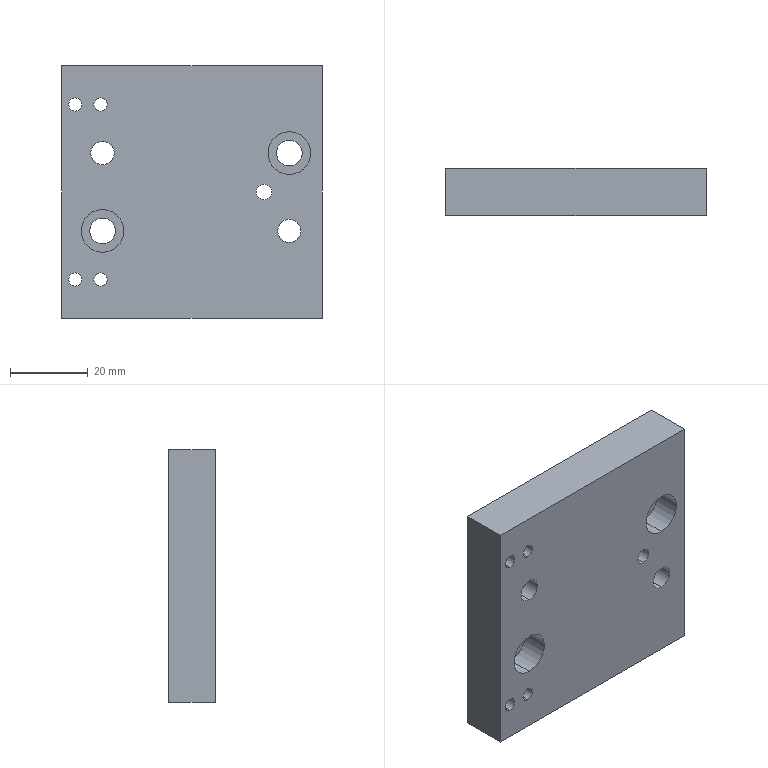Part | SolidWorks | features HoleWzd 3, Extrusion 1 | 1 solid | 42 faces | box 67 x 12 x 65 mm | volume 49086 mm3 | cylinder 30 | plane 12 | commonest cylinder face diameters 6 x12 3.4 x8 6.6 x4 11 x4 4 x2
STEP:
#1=CARTESIAN_POINT('',(25.,6.,-7.));
#2=VERTEX_POINT('',#1);
#3=CARTESIAN_POINT('',(25.,6.,-13.));
#4=VERTEX_POINT('',#3);
#5=CARTESIAN_POINT('',(25.,6.,-10.));
#6=DIRECTION('',(0.,-1.,0.));
#7=DIRECTION('',(0.,0.,-1.));
#8=AXIS2_PLACEMENT_3D('',#5,#6,#7);
#9=CIRCLE('',#8,3.);
#10=EDGE_CURVE('',#2,#4,#9,.T.);
#11=ORIENTED_EDGE('',*,*,#10,.F.);
#12=CARTESIAN_POINT('',(25.,-6.,-7.));
#13=VERTEX_POINT('',#12);
#14=CARTESIAN_POINT('',(25.,-6.,-7.));
#15=DIRECTION('',(0.,-1.,0.));
#16=VECTOR('',#15,1000.);
#17=LINE('',#14,#16);
#18=EDGE_CURVE('',#2,#13,#17,.T.);
#19=ORIENTED_EDGE('',*,*,#18,.T.);
#20=CARTESIAN_POINT('',(25.,-6.,-13.));
#21=VERTEX_POINT('',#20);
#22=CARTESIAN_POINT('',(25.,-6.,-10.));
#23=DIRECTION('',(0.,-1.,0.));
#24=DIRECTION('',(0.,0.,-1.));
#25=AXIS2_PLACEMENT_3D('',#22,#23,#24);
#26=CIRCLE('',#25,3.);
#27=EDGE_CURVE('',#13,#21,#26,.T.);
#28=ORIENTED_EDGE('',*,*,#27,.T.);
#29=CARTESIAN_POINT('',(25.,-6.,-13.));
#30=DIRECTION('',(0.,-1.,0.));
#31=VECTOR('',#30,1000.);
#32=LINE('',#29,#31);
#33=EDGE_CURVE('',#4,#21,#32,.T.);
#34=ORIENTED_EDGE('',*,*,#33,.F.);
#35=EDGE_LOOP('',(#11,#19,#28,#34));
#36=FACE_OUTER_BOUND('',#35,.T.);
#37=CARTESIAN_POINT('',(25.,-6.,-10.));
#38=DIRECTION('',(0.,-1.,0.));
#39=DIRECTION('',(0.,0.,-1.));
#40=AXIS2_PLACEMENT_3D('',#37,#38,#39);
#41=CYLINDRICAL_SURFACE('',#40,3.);
#42=ADVANCED_FACE('',(#36),#41,.F.);
#43=CARTESIAN_POINT('',(-23.,6.,13.));
#44=VERTEX_POINT('',#43);
#45=CARTESIAN_POINT('',(-23.,6.,7.));
#46=VERTEX_POINT('',#45);
#47=CARTESIAN_POINT('',(-23.,6.,10.));
#48=DIRECTION('',(0.,-1.,0.));
#49=DIRECTION('',(0.,0.,-1.));
#50=AXIS2_PLACEMENT_3D('',#47,#48,#49);
#51=CIRCLE('',#50,3.);
#52=EDGE_CURVE('',#44,#46,#51,.T.);
#53=ORIENTED_EDGE('',*,*,#52,.F.);
#54=CARTESIAN_POINT('',(-23.,-6.,13.));
#55=VERTEX_POINT('',#54);
#56=CARTESIAN_POINT('',(-23.,-6.,13.));
#57=DIRECTION('',(0.,-1.,0.));
#58=VECTOR('',#57,1000.);
#59=LINE('',#56,#58);
#60=EDGE_CURVE('',#44,#55,#59,.T.);
#61=ORIENTED_EDGE('',*,*,#60,.T.);
#62=CARTESIAN_POINT('',(-23.,-6.,7.));
#63=VERTEX_POINT('',#62);
#64=CARTESIAN_POINT('',(-23.,-6.,10.));
#65=DIRECTION('',(0.,-1.,0.));
#66=DIRECTION('',(0.,0.,-1.));
#67=AXIS2_PLACEMENT_3D('',#64,#65,#66);
#68=CIRCLE('',#67,3.);
#69=EDGE_CURVE('',#55,#63,#68,.T.);
#70=ORIENTED_EDGE('',*,*,#69,.T.);
#71=CARTESIAN_POINT('',(-23.,-6.,7.));
#72=DIRECTION('',(0.,-1.,0.));
#73=VECTOR('',#72,1000.);
#74=LINE('',#71,#73);
#75=EDGE_CURVE('',#46,#63,#74,.T.);
#76=ORIENTED_EDGE('',*,*,#75,.F.);
#77=EDGE_LOOP('',(#53,#61,#70,#76));
#78=FACE_OUTER_BOUND('',#77,.T.);
#79=CARTESIAN_POINT('',(-23.,-6.,10.));
#80=DIRECTION('',(0.,-1.,0.));
#81=DIRECTION('',(0.,0.,-1.));
#82=AXIS2_PLACEMENT_3D('',#79,#80,#81);
#83=CYLINDRICAL_SURFACE('',#82,3.);
#84=ADVANCED_FACE('',(#78),#83,.F.);
#85=CARTESIAN_POINT('',(-23.,0.8,-4.5));
#86=VERTEX_POINT('',#85);
#87=CARTESIAN_POINT('',(-23.,0.8,-15.5));
#88=VERTEX_POINT('',#87);
#89=CARTESIAN_POINT('',(-23.,0.8,-10.));
#90=DIRECTION('',(0.,-1.,0.));
#91=DIRECTION('',(0.,0.,-1.));
#92=AXIS2_PLACEMENT_3D('',#89,#90,#91);
#93=CIRCLE('',#92,5.5);
#94=EDGE_CURVE('',#86,#88,#93,.T.);
#95=ORIENTED_EDGE('',*,*,#94,.F.);
#96=CARTESIAN_POINT('',(-23.,-6.,-4.5));
#97=VERTEX_POINT('',#96);
#98=CARTESIAN_POINT('',(-23.,-6.,-4.5));
#99=DIRECTION('',(0.,-1.,0.));
#100=VECTOR('',#99,1000.);
#101=LINE('',#98,#100);
#102=EDGE_CURVE('',#86,#97,#101,.T.);
#103=ORIENTED_EDGE('',*,*,#102,.T.);
#104=CARTESIAN_POINT('',(-23.,-6.,-15.5));
#105=VERTEX_POINT('',#104);
#106=CARTESIAN_POINT('',(-23.,-6.,-10.));
#107=DIRECTION('',(0.,-1.,0.));
#108=DIRECTION('',(0.,0.,-1.));
#109=AXIS2_PLACEMENT_3D('',#106,#107,#108);
#110=CIRCLE('',#109,5.5);
#111=EDGE_CURVE('',#97,#105,#110,.T.);
#112=ORIENTED_EDGE('',*,*,#111,.T.);
#113=CARTESIAN_POINT('',(-23.,-6.,-15.5));
#114=DIRECTION('',(0.,-1.,0.));
#115=VECTOR('',#114,1000.);
#116=LINE('',#113,#115);
#117=EDGE_CURVE('',#88,#105,#116,.T.);
#118=ORIENTED_EDGE('',*,*,#117,.F.);
#119=EDGE_LOOP('',(#95,#103,#112,#118));
#120=FACE_OUTER_BOUND('',#119,.T.);
#121=CARTESIAN_POINT('',(-23.,-6.,-10.));
#122=DIRECTION('',(0.,-1.,0.));
#123=DIRECTION('',(0.,0.,-1.));
#124=AXIS2_PLACEMENT_3D('',#121,#122,#123);
#125=CYLINDRICAL_SURFACE('',#124,5.5);
#126=ADVANCED_FACE('',(#120),#125,.F.);
#127=CARTESIAN_POINT('',(-23.,6.,-6.7));
#128=VERTEX_POINT('',#127);
#129=CARTESIAN_POINT('',(-23.,6.,-13.3));
#130=VERTEX_POINT('',#129);
#131=CARTESIAN_POINT('',(-23.,6.,-10.));
#132=DIRECTION('',(0.,-1.,0.));
#133=DIRECTION('',(0.,0.,-1.));
#134=AXIS2_PLACEMENT_3D('',#131,#132,#133);
#135=CIRCLE('',#134,3.3);
#136=EDGE_CURVE('',#128,#130,#135,.T.);
#137=ORIENTED_EDGE('',*,*,#136,.F.);
#138=CARTESIAN_POINT('',(-23.,0.8,-6.7));
#139=VERTEX_POINT('',#138);
#140=CARTESIAN_POINT('',(-23.,-6.,-6.7));
#141=DIRECTION('',(0.,-1.,0.));
#142=VECTOR('',#141,1000.);
#143=LINE('',#140,#142);
#144=EDGE_CURVE('',#128,#139,#143,.T.);
#145=ORIENTED_EDGE('',*,*,#144,.T.);
#146=CARTESIAN_POINT('',(-23.,0.8,-13.3));
#147=VERTEX_POINT('',#146);
#148=CARTESIAN_POINT('',(-23.,0.8,-10.));
#149=DIRECTION('',(0.,-1.,0.));
#150=DIRECTION('',(0.,0.,-1.));
#151=AXIS2_PLACEMENT_3D('',#148,#149,#150);
#152=CIRCLE('',#151,3.3);
#153=EDGE_CURVE('',#139,#147,#152,.T.);
#154=ORIENTED_EDGE('',*,*,#153,.T.);
#155=CARTESIAN_POINT('',(-23.,-6.,-13.3));
#156=DIRECTION('',(0.,-1.,0.));
#157=VECTOR('',#156,1000.);
#158=LINE('',#155,#157);
#159=EDGE_CURVE('',#130,#147,#158,.T.);
#160=ORIENTED_EDGE('',*,*,#159,.F.);
#161=EDGE_LOOP('',(#137,#145,#154,#160));
#162=FACE_OUTER_BOUND('',#161,.T.);
#163=CARTESIAN_POINT('',(-23.,-6.,-10.));
#164=DIRECTION('',(0.,-1.,0.));
#165=DIRECTION('',(0.,0.,-1.));
#166=AXIS2_PLACEMENT_3D('',#163,#164,#165);
#167=CYLINDRICAL_SURFACE('',#166,3.3);
#168=ADVANCED_FACE('',(#162),#167,.F.);
#169=CARTESIAN_POINT('',(25.,0.8,15.5));
#170=VERTEX_POINT('',#169);
#171=CARTESIAN_POINT('',(25.,0.8,4.5));
#172=VERTEX_POINT('',#171);
#173=CARTESIAN_POINT('',(25.,0.8,10.));
#174=DIRECTION('',(0.,-1.,0.));
#175=DIRECTION('',(0.,0.,-1.));
#176=AXIS2_PLACEMENT_3D('',#173,#174,#175);
#177=CIRCLE('',#176,5.5);
#178=EDGE_CURVE('',#170,#172,#177,.T.);
#179=ORIENTED_EDGE('',*,*,#178,.F.);
#180=CARTESIAN_POINT('',(25.,-6.,15.5));
#181=VERTEX_POINT('',#180);
#182=CARTESIAN_POINT('',(25.,-6.,15.5));
#183=DIRECTION('',(0.,-1.,0.));
#184=VECTOR('',#183,1000.);
#185=LINE('',#182,#184);
#186=EDGE_CURVE('',#170,#181,#185,.T.);
#187=ORIENTED_EDGE('',*,*,#186,.T.);
#188=CARTESIAN_POINT('',(25.,-6.,4.5));
#189=VERTEX_POINT('',#188);
#190=CARTESIAN_POINT('',(25.,-6.,10.));
#191=DIRECTION('',(0.,-1.,0.));
#192=DIRECTION('',(0.,0.,-1.));
#193=AXIS2_PLACEMENT_3D('',#190,#191,#192);
#194=CIRCLE('',#193,5.5);
#195=EDGE_CURVE('',#181,#189,#194,.T.);
#196=ORIENTED_EDGE('',*,*,#195,.T.);
#197=CARTESIAN_POINT('',(25.,-6.,4.5));
#198=DIRECTION('',(0.,-1.,0.));
#199=VECTOR('',#198,1000.);
#200=LINE('',#197,#199);
#201=EDGE_CURVE('',#172,#189,#200,.T.);
#202=ORIENTED_EDGE('',*,*,#201,.F.);
#203=EDGE_LOOP('',(#179,#187,#196,#202));
#204=FACE_OUTER_BOUND('',#203,.T.);
#205=CARTESIAN_POINT('',(25.,-6.,10.));
#206=DIRECTION('',(0.,-1.,0.));
#207=DIRECTION('',(0.,0.,-1.));
#208=AXIS2_PLACEMENT_3D('',#205,#206,#207);
#209=CYLINDRICAL_SURFACE('',#208,5.5);
#210=ADVANCED_FACE('',(#204),#209,.F.);
#211=CARTESIAN_POINT('',(25.,6.,13.3));
#212=VERTEX_POINT('',#211);
#213=CARTESIAN_POINT('',(25.,6.,6.7));
#214=VERTEX_POINT('',#213);
#215=CARTESIAN_POINT('',(25.,6.,10.));
#216=DIRECTION('',(0.,-1.,0.));
#217=DIRECTION('',(0.,0.,-1.));
#218=AXIS2_PLACEMENT_3D('',#215,#216,#217);
#219=CIRCLE('',#218,3.3);
#220=EDGE_CURVE('',#212,#214,#219,.T.);
#221=ORIENTED_EDGE('',*,*,#220,.F.);
#222=CARTESIAN_POINT('',(25.,0.8,13.3));
#223=VERTEX_POINT('',#222);
#224=CARTESIAN_POINT('',(25.,-6.,13.3));
#225=DIRECTION('',(0.,-1.,0.));
#226=VECTOR('',#225,1000.);
#227=LINE('',#224,#226);
#228=EDGE_CURVE('',#212,#223,#227,.T.);
#229=ORIENTED_EDGE('',*,*,#228,.T.);
#230=CARTESIAN_POINT('',(25.,0.8,6.7));
#231=VERTEX_POINT('',#230);
#232=CARTESIAN_POINT('',(25.,0.8,10.));
#233=DIRECTION('',(0.,-1.,0.));
#234=DIRECTION('',(0.,0.,-1.));
#235=AXIS2_PLACEMENT_3D('',#232,#233,#234);
#236=CIRCLE('',#235,3.3);
#237=EDGE_CURVE('',#223,#231,#236,.T.);
#238=ORIENTED_EDGE('',*,*,#237,.T.);
#239=CARTESIAN_POINT('',(25.,-6.,6.7));
#240=DIRECTION('',(0.,-1.,0.));
#241=VECTOR('',#240,1000.);
#242=LINE('',#239,#241);
#243=EDGE_CURVE('',#214,#231,#242,.T.);
#244=ORIENTED_EDGE('',*,*,#243,.F.);
#245=EDGE_LOOP('',(#221,#229,#238,#244));
#246=FACE_OUTER_BOUND('',#245,.T.);
#247=CARTESIAN_POINT('',(25.,-6.,10.));
#248=DIRECTION('',(0.,-1.,0.));
#249=DIRECTION('',(0.,0.,-1.));
#250=AXIS2_PLACEMENT_3D('',#247,#248,#249);
#251=CYLINDRICAL_SURFACE('',#250,3.3);
#252=ADVANCED_FACE('',(#246),#251,.F.);
#253=CARTESIAN_POINT('',(-30.,2.6,19.5));
#254=VERTEX_POINT('',#253);
#255=CARTESIAN_POINT('',(-30.,2.6,25.5));
#256=VERTEX_POINT('',#255);
#257=CARTESIAN_POINT('',(-30.,2.6,22.5));
#258=DIRECTION('',(0.,1.,0.));
#259=DIRECTION('',(0.,0.,1.));
#260=AXIS2_PLACEMENT_3D('',#257,#258,#259);
#261=CIRCLE('',#260,3.);
#262=EDGE_CURVE('',#254,#256,#261,.T.);
#263=ORIENTED_EDGE('',*,*,#262,.F.);
#264=CARTESIAN_POINT('',(-30.,6.,19.5));
#265=VERTEX_POINT('',#264);
#266=CARTESIAN_POINT('',(-30.,6.,19.5));
#267=DIRECTION('',(0.,1.,0.));
#268=VECTOR('',#267,1000.);
#269=LINE('',#266,#268);
#270=EDGE_CURVE('',#254,#265,#269,.T.);
#271=ORIENTED_EDGE('',*,*,#270,.T.);
#272=CARTESIAN_POINT('',(-30.,6.,25.5));
#273=VERTEX_POINT('',#272);
#274=CARTESIAN_POINT('',(-30.,6.,22.5));
#275=DIRECTION('',(0.,1.,0.));
#276=DIRECTION('',(0.,0.,1.));
#277=AXIS2_PLACEMENT_3D('',#274,#275,#276);
#278=CIRCLE('',#277,3.);
#279=EDGE_CURVE('',#265,#273,#278,.T.);
#280=ORIENTED_EDGE('',*,*,#279,.T.);
#281=CARTESIAN_POINT('',(-30.,6.,25.5));
#282=DIRECTION('',(0.,1.,0.));
#283=VECTOR('',#282,1000.);
#284=LINE('',#281,#283);
#285=EDGE_CURVE('',#256,#273,#284,.T.);
#286=ORIENTED_EDGE('',*,*,#285,.F.);
#287=EDGE_LOOP('',(#263,#271,#280,#286));
#288=FACE_OUTER_BOUND('',#287,.T.);
#289=CARTESIAN_POINT('',(-30.,6.,22.5));
#290=DIRECTION('',(0.,1.,0.));
#291=DIRECTION('',(0.,0.,1.));
#292=AXIS2_PLACEMENT_3D('',#289,#290,#291);
#293=CYLINDRICAL_SURFACE('',#292,3.);
#294=ADVANCED_FACE('',(#288),#293,.F.);
#295=CARTESIAN_POINT('',(-30.,-6.,20.8));
#296=VERTEX_POINT('',#295);
#297=CARTESIAN_POINT('',(-30.,-6.,24.2));
#298=VERTEX_POINT('',#297);
#299=CARTESIAN_POINT('',(-30.,-6.,22.5));
#300=DIRECTION('',(0.,1.,0.));
#301=DIRECTION('',(0.,0.,1.));
#302=AXIS2_PLACEMENT_3D('',#299,#300,#301);
#303=CIRCLE('',#302,1.7);
#304=EDGE_CURVE('',#296,#298,#303,.T.);
#305=ORIENTED_EDGE('',*,*,#304,.F.);
#306=CARTESIAN_POINT('',(-30.,2.6,20.8));
#307=VERTEX_POINT('',#306);
#308=CARTESIAN_POINT('',(-30.,6.,20.8));
#309=DIRECTION('',(0.,1.,0.));
#310=VECTOR('',#309,1000.);
#311=LINE('',#308,#310);
#312=EDGE_CURVE('',#296,#307,#311,.T.);
#313=ORIENTED_EDGE('',*,*,#312,.T.);
#314=CARTESIAN_POINT('',(-30.,2.6,24.2));
#315=VERTEX_POINT('',#314);
#316=CARTESIAN_POINT('',(-30.,2.6,22.5));
#317=DIRECTION('',(0.,1.,0.));
#318=DIRECTION('',(0.,0.,1.));
#319=AXIS2_PLACEMENT_3D('',#316,#317,#318);
#320=CIRCLE('',#319,1.7);
#321=EDGE_CURVE('',#307,#315,#320,.T.);
#322=ORIENTED_EDGE('',*,*,#321,.T.);
#323=CARTESIAN_POINT('',(-30.,6.,24.2));
#324=DIRECTION('',(0.,1.,0.));
#325=VECTOR('',#324,1000.);
#326=LINE('',#323,#325);
#327=EDGE_CURVE('',#298,#315,#326,.T.);
#328=ORIENTED_EDGE('',*,*,#327,.F.);
#329=EDGE_LOOP('',(#305,#313,#322,#328));
#330=FACE_OUTER_BOUND('',#329,.T.);
#331=CARTESIAN_POINT('',(-30.,6.,22.5));
#332=DIRECTION('',(0.,1.,0.));
#333=DIRECTION('',(0.,0.,1.));
#334=AXIS2_PLACEMENT_3D('',#331,#332,#333);
#335=CYLINDRICAL_SURFACE('',#334,1.7);
#336=ADVANCED_FACE('',(#330),#335,.F.);
#337=CARTESIAN_POINT('',(-23.5,2.6,19.5));
#338=VERTEX_POINT('',#337);
#339=CARTESIAN_POINT('',(-23.5,2.6,25.5));
#340=VERTEX_POINT('',#339);
#341=CARTESIAN_POINT('',(-23.5,2.6,22.5));
#342=DIRECTION('',(0.,1.,0.));
#343=DIRECTION('',(0.,0.,1.));
#344=AXIS2_PLACEMENT_3D('',#341,#342,#343);
#345=CIRCLE('',#344,3.);
#346=EDGE_CURVE('',#338,#340,#345,.T.);
#347=ORIENTED_EDGE('',*,*,#346,.F.);
#348=CARTESIAN_POINT('',(-23.5,6.,19.5));
#349=VERTEX_POINT('',#348);
#350=CARTESIAN_POINT('',(-23.5,6.,19.5));
#351=DIRECTION('',(0.,1.,0.));
#352=VECTOR('',#351,1000.);
#353=LINE('',#350,#352);
#354=EDGE_CURVE('',#338,#349,#353,.T.);
#355=ORIENTED_EDGE('',*,*,#354,.T.);
#356=CARTESIAN_POINT('',(-23.5,6.,25.5));
#357=VERTEX_POINT('',#356);
#358=CARTESIAN_POINT('',(-23.5,6.,22.5));
#359=DIRECTION('',(0.,1.,0.));
#360=DIRECTION('',(0.,0.,1.));
#361=AXIS2_PLACEMENT_3D('',#358,#359,#360);
#362=CIRCLE('',#361,3.);
#363=EDGE_CURVE('',#349,#357,#362,.T.);
#364=ORIENTED_EDGE('',*,*,#363,.T.);
#365=CARTESIAN_POINT('',(-23.5,6.,25.5));
#366=DIRECTION('',(0.,1.,0.));
#367=VECTOR('',#366,1000.);
#368=LINE('',#365,#367);
#369=EDGE_CURVE('',#340,#357,#368,.T.);
#370=ORIENTED_EDGE('',*,*,#369,.F.);
#371=EDGE_LOOP('',(#347,#355,#364,#370));
#372=FACE_OUTER_BOUND('',#371,.T.);
#373=CARTESIAN_POINT('',(-23.5,6.,22.5));
#374=DIRECTION('',(0.,1.,0.));
#375=DIRECTION('',(0.,0.,1.));
#376=AXIS2_PLACEMENT_3D('',#373,#374,#375);
#377=CYLINDRICAL_SURFACE('',#376,3.);
#378=ADVANCED_FACE('',(#372),#377,.F.);
#379=CARTESIAN_POINT('',(-23.5,-6.,20.8));
#380=VERTEX_POINT('',#379);
#381=CARTESIAN_POINT('',(-23.5,-6.,24.2));
#382=VERTEX_POINT('',#381);
#383=CARTESIAN_POINT('',(-23.5,-6.,22.5));
#384=DIRECTION('',(0.,1.,0.));
#385=DIRECTION('',(0.,0.,1.));
#386=AXIS2_PLACEMENT_3D('',#383,#384,#385);
#387=CIRCLE('',#386,1.7);
#388=EDGE_CURVE('',#380,#382,#387,.T.);
#389=ORIENTED_EDGE('',*,*,#388,.F.);
#390=CARTESIAN_POINT('',(-23.5,2.6,20.8));
#391=VERTEX_POINT('',#390);
#392=CARTESIAN_POINT('',(-23.5,6.,20.8));
#393=DIRECTION('',(0.,1.,0.));
#394=VECTOR('',#393,1000.);
#395=LINE('',#392,#394);
#396=EDGE_CURVE('',#380,#391,#395,.T.);
#397=ORIENTED_EDGE('',*,*,#396,.T.);
#398=CARTESIAN_POINT('',(-23.5,2.6,24.2));
#399=VERTEX_POINT('',#398);
#400=CARTESIAN_POINT('',(-23.5,2.6,22.5));
#401=DIRECTION('',(0.,1.,0.));
#402=DIRECTION('',(0.,0.,1.));
#403=AXIS2_PLACEMENT_3D('',#400,#401,#402);
#404=CIRCLE('',#403,1.7);
#405=EDGE_CURVE('',#391,#399,#404,.T.);
#406=ORIENTED_EDGE('',*,*,#405,.T.);
#407=CARTESIAN_POINT('',(-23.5,6.,24.2));
#408=DIRECTION('',(0.,1.,0.));
#409=VECTOR('',#408,1000.);
#410=LINE('',#407,#409);
#411=EDGE_CURVE('',#382,#399,#410,.T.);
#412=ORIENTED_EDGE('',*,*,#411,.F.);
#413=EDGE_LOOP('',(#389,#397,#406,#412));
#414=FACE_OUTER_BOUND('',#413,.T.);
#415=CARTESIAN_POINT('',(-23.5,6.,22.5));
#416=DIRECTION('',(0.,1.,0.));
#417=DIRECTION('',(0.,0.,1.));
#418=AXIS2_PLACEMENT_3D('',#415,#416,#417);
#419=CYLINDRICAL_SURFACE('',#418,1.7);
#420=ADVANCED_FACE('',(#414),#419,.F.);
#421=CARTESIAN_POINT('',(-23.5,2.6,-25.5));
#422=VERTEX_POINT('',#421);
#423=CARTESIAN_POINT('',(-23.5,2.6,-19.5));
#424=VERTEX_POINT('',#423);
#425=CARTESIAN_POINT('',(-23.5,2.6,-22.5));
#426=DIRECTION('',(0.,1.,0.));
#427=DIRECTION('',(0.,0.,1.));
#428=AXIS2_PLACEMENT_3D('',#425,#426,#427);
#429=CIRCLE('',#428,3.);
#430=EDGE_CURVE('',#422,#424,#429,.T.);
#431=ORIENTED_EDGE('',*,*,#430,.F.);
#432=CARTESIAN_POINT('',(-23.5,6.,-25.5));
#433=VERTEX_POINT('',#432);
#434=CARTESIAN_POINT('',(-23.5,6.,-25.5));
#435=DIRECTION('',(0.,1.,0.));
#436=VECTOR('',#435,1000.);
#437=LINE('',#434,#436);
#438=EDGE_CURVE('',#422,#433,#437,.T.);
#439=ORIENTED_EDGE('',*,*,#438,.T.);
#440=CARTESIAN_POINT('',(-23.5,6.,-19.5));
#441=VERTEX_POINT('',#440);
#442=CARTESIAN_POINT('',(-23.5,6.,-22.5));
#443=DIRECTION('',(0.,1.,0.));
#444=DIRECTION('',(0.,0.,1.));
#445=AXIS2_PLACEMENT_3D('',#442,#443,#444);
#446=CIRCLE('',#445,3.);
#447=EDGE_CURVE('',#433,#441,#446,.T.);
#448=ORIENTED_EDGE('',*,*,#447,.T.);
#449=CARTESIAN_POINT('',(-23.5,6.,-19.5));
#450=DIRECTION('',(0.,1.,0.));
#451=VECTOR('',#450,1000.);
#452=LINE('',#449,#451);
#453=EDGE_CURVE('',#424,#441,#452,.T.);
#454=ORIENTED_EDGE('',*,*,#453,.F.);
#455=EDGE_LOOP('',(#431,#439,#448,#454));
#456=FACE_OUTER_BOUND('',#455,.T.);
#457=CARTESIAN_POINT('',(-23.5,6.,-22.5));
#458=DIRECTION('',(0.,1.,0.));
#459=DIRECTION('',(0.,0.,1.));
#460=AXIS2_PLACEMENT_3D('',#457,#458,#459);
#461=CYLINDRICAL_SURFACE('',#460,3.);
#462=ADVANCED_FACE('',(#456),#461,.F.);
#463=CARTESIAN_POINT('',(-23.5,-6.,-24.2));
#464=VERTEX_POINT('',#463);
#465=CARTESIAN_POINT('',(-23.5,-6.,-20.8));
#466=VERTEX_POINT('',#465);
#467=CARTESIAN_POINT('',(-23.5,-6.,-22.5));
#468=DIRECTION('',(0.,1.,0.));
#469=DIRECTION('',(0.,0.,1.));
#470=AXIS2_PLACEMENT_3D('',#467,#468,#469);
#471=CIRCLE('',#470,1.7);
#472=EDGE_CURVE('',#464,#466,#471,.T.);
#473=ORIENTED_EDGE('',*,*,#472,.F.);
#474=CARTESIAN_POINT('',(-23.5,2.6,-24.2));
#475=VERTEX_POINT('',#474);
#476=CARTESIAN_POINT('',(-23.5,6.,-24.2));
#477=DIRECTION('',(0.,1.,0.));
#478=VECTOR('',#477,1000.);
#479=LINE('',#476,#478);
#480=EDGE_CURVE('',#464,#475,#479,.T.);
#481=ORIENTED_EDGE('',*,*,#480,.T.);
#482=CARTESIAN_POINT('',(-23.5,2.6,-20.8));
#483=VERTEX_POINT('',#482);
#484=CARTESIAN_POINT('',(-23.5,2.6,-22.5));
#485=DIRECTION('',(0.,1.,0.));
#486=DIRECTION('',(0.,0.,1.));
#487=AXIS2_PLACEMENT_3D('',#484,#485,#486);
#488=CIRCLE('',#487,1.7);
#489=EDGE_CURVE('',#475,#483,#488,.T.);
#490=ORIENTED_EDGE('',*,*,#489,.T.);
#491=CARTESIAN_POINT('',(-23.5,6.,-20.8));
#492=DIRECTION('',(0.,1.,0.));
#493=VECTOR('',#492,1000.);
#494=LINE('',#491,#493);
#495=EDGE_CURVE('',#466,#483,#494,.T.);
#496=ORIENTED_EDGE('',*,*,#495,.F.);
#497=EDGE_LOOP('',(#473,#481,#490,#496));
#498=FACE_OUTER_BOUND('',#497,.T.);
#499=CARTESIAN_POINT('',(-23.5,6.,-22.5));
#500=DIRECTION('',(0.,1.,0.));
#501=DIRECTION('',(0.,0.,1.));
#502=AXIS2_PLACEMENT_3D('',#499,#500,#501);
#503=CYLINDRICAL_SURFACE('',#502,1.7);
#504=ADVANCED_FACE('',(#498),#503,.F.);
#505=CARTESIAN_POINT('',(-30.,2.6,-25.5));
#506=VERTEX_POINT('',#505);
#507=CARTESIAN_POINT('',(-30.,2.6,-19.5));
#508=VERTEX_POINT('',#507);
#509=CARTESIAN_POINT('',(-30.,2.6,-22.5));
#510=DIRECTION('',(0.,1.,0.));
#511=DIRECTION('',(0.,0.,1.));
#512=AXIS2_PLACEMENT_3D('',#509,#510,#511);
#513=CIRCLE('',#512,3.);
#514=EDGE_CURVE('',#506,#508,#513,.T.);
#515=ORIENTED_EDGE('',*,*,#514,.F.);
#516=CARTESIAN_POINT('',(-30.,6.,-25.5));
#517=VERTEX_POINT('',#516);
#518=CARTESIAN_POINT('',(-30.,6.,-25.5));
#519=DIRECTION('',(0.,1.,0.));
#520=VECTOR('',#519,1000.);
#521=LINE('',#518,#520);
#522=EDGE_CURVE('',#506,#517,#521,.T.);
#523=ORIENTED_EDGE('',*,*,#522,.T.);
#524=CARTESIAN_POINT('',(-30.,6.,-19.5));
#525=VERTEX_POINT('',#524);
#526=CARTESIAN_POINT('',(-30.,6.,-22.5));
#527=DIRECTION('',(0.,1.,0.));
#528=DIRECTION('',(0.,0.,1.));
#529=AXIS2_PLACEMENT_3D('',#526,#527,#528);
#530=CIRCLE('',#529,3.);
#531=EDGE_CURVE('',#517,#525,#530,.T.);
#532=ORIENTED_EDGE('',*,*,#531,.T.);
#533=CARTESIAN_POINT('',(-30.,6.,-19.5));
#534=DIRECTION('',(0.,1.,0.));
#535=VECTOR('',#534,1000.);
#536=LINE('',#533,#535);
#537=EDGE_CURVE('',#508,#525,#536,.T.);
#538=ORIENTED_EDGE('',*,*,#537,.F.);
#539=EDGE_LOOP('',(#515,#523,#532,#538));
#540=FACE_OUTER_BOUND('',#539,.T.);
#541=CARTESIAN_POINT('',(-30.,6.,-22.5));
#542=DIRECTION('',(0.,1.,0.));
#543=DIRECTION('',(0.,0.,1.));
#544=AXIS2_PLACEMENT_3D('',#541,#542,#543);
#545=CYLINDRICAL_SURFACE('',#544,3.);
#546=ADVANCED_FACE('',(#540),#545,.F.);
#547=CARTESIAN_POINT('',(-30.,-6.,-24.2));
#548=VERTEX_POINT('',#547);
#549=CARTESIAN_POINT('',(-30.,-6.,-20.8));
#550=VERTEX_POINT('',#549);
#551=CARTESIAN_POINT('',(-30.,-6.,-22.5));
#552=DIRECTION('',(0.,1.,0.));
#553=DIRECTION('',(0.,0.,1.));
#554=AXIS2_PLACEMENT_3D('',#551,#552,#553);
#555=CIRCLE('',#554,1.7);
#556=EDGE_CURVE('',#548,#550,#555,.T.);
#557=ORIENTED_EDGE('',*,*,#556,.F.);
#558=CARTESIAN_POINT('',(-30.,2.6,-24.2));
#559=VERTEX_POINT('',#558);
#560=CARTESIAN_POINT('',(-30.,6.,-24.2));
#561=DIRECTION('',(0.,1.,0.));
#562=VECTOR('',#561,1000.);
#563=LINE('',#560,#562);
#564=EDGE_CURVE('',#548,#559,#563,.T.);
#565=ORIENTED_EDGE('',*,*,#564,.T.);
#566=CARTESIAN_POINT('',(-30.,2.6,-20.8));
#567=VERTEX_POINT('',#566);
#568=CARTESIAN_POINT('',(-30.,2.6,-22.5));
#569=DIRECTION('',(0.,1.,0.));
#570=DIRECTION('',(0.,0.,1.));
#571=AXIS2_PLACEMENT_3D('',#568,#569,#570);
#572=CIRCLE('',#571,1.7);
#573=EDGE_CURVE('',#559,#567,#572,.T.);
#574=ORIENTED_EDGE('',*,*,#573,.T.);
#575=CARTESIAN_POINT('',(-30.,6.,-20.8));
#576=DIRECTION('',(0.,1.,0.));
#577=VECTOR('',#576,1000.);
#578=LINE('',#575,#577);
#579=EDGE_CURVE('',#550,#567,#578,.T.);
#580=ORIENTED_EDGE('',*,*,#579,.F.);
#581=EDGE_LOOP('',(#557,#565,#574,#580));
#582=FACE_OUTER_BOUND('',#581,.T.);
#583=CARTESIAN_POINT('',(-30.,6.,-22.5));
#584=DIRECTION('',(0.,1.,0.));
#585=DIRECTION('',(0.,0.,1.));
#586=AXIS2_PLACEMENT_3D('',#583,#584,#585);
#587=CYLINDRICAL_SURFACE('',#586,1.7);
#588=ADVANCED_FACE('',(#582),#587,.F.);
#589=CARTESIAN_POINT('',(18.5,6.,-2.));
#590=VERTEX_POINT('',#589);
#591=CARTESIAN_POINT('',(18.5,6.,2.));
#592=VERTEX_POINT('',#591);
#593=CARTESIAN_POINT('',(18.5,6.,0.));
#594=DIRECTION('',(0.,1.,0.));
#595=DIRECTION('',(0.,0.,1.));
#596=AXIS2_PLACEMENT_3D('',#593,#594,#595);
#597=CIRCLE('',#596,2.);
#598=EDGE_CURVE('',#590,#592,#597,.T.);
#599=ORIENTED_EDGE('',*,*,#598,.T.);
#600=CARTESIAN_POINT('',(18.5,-6.,2.));
#601=VERTEX_POINT('',#600);
#602=CARTESIAN_POINT('',(18.5,6.,2.));
#603=DIRECTION('',(0.,-1.,0.));
#604=VECTOR('',#603,1000.);
#605=LINE('',#602,#604);
#606=EDGE_CURVE('',#592,#601,#605,.T.);
#607=ORIENTED_EDGE('',*,*,#606,.T.);
#608=CARTESIAN_POINT('',(18.5,-6.,-2.));
#609=VERTEX_POINT('',#608);
#610=CARTESIAN_POINT('',(18.5,-6.,0.));
#611=DIRECTION('',(0.,1.,0.));
#612=DIRECTION('',(0.,0.,1.));
#613=AXIS2_PLACEMENT_3D('',#610,#611,#612);
#614=CIRCLE('',#613,2.);
#615=EDGE_CURVE('',#609,#601,#614,.T.);
#616=ORIENTED_EDGE('',*,*,#615,.F.);
#617=CARTESIAN_POINT('',(18.5,6.,-2.));
#618=DIRECTION('',(0.,-1.,0.));
#619=VECTOR('',#618,1000.);
#620=LINE('',#617,#619);
#621=EDGE_CURVE('',#590,#609,#620,.T.);
#622=ORIENTED_EDGE('',*,*,#621,.F.);
#623=EDGE_LOOP('',(#599,#607,#616,#622));
#624=FACE_OUTER_BOUND('',#623,.T.);
#625=CARTESIAN_POINT('',(18.5,6.,0.));
#626=DIRECTION('',(0.,-1.,0.));
#627=DIRECTION('',(0.,0.,-1.));
#628=AXIS2_PLACEMENT_3D('',#625,#626,#627);
#629=CYLINDRICAL_SURFACE('',#628,2.);
#630=ADVANCED_FACE('',(#624),#629,.F.);
#631=CARTESIAN_POINT('',(25.,6.,-10.));
#632=DIRECTION('',(0.,-1.,0.));
#633=DIRECTION('',(0.,0.,-1.));
#634=AXIS2_PLACEMENT_3D('',#631,#632,#633);
#635=CIRCLE('',#634,3.);
#636=EDGE_CURVE('',#4,#2,#635,.T.);
#637=ORIENTED_EDGE('',*,*,#636,.T.);
#638=ORIENTED_EDGE('',*,*,#10,.T.);
#639=EDGE_LOOP('',(#637,#638));
#640=FACE_BOUND('',#639,.T.);
#641=CARTESIAN_POINT('',(-23.,6.,10.));
#642=DIRECTION('',(0.,-1.,0.));
#643=DIRECTION('',(0.,0.,-1.));
#644=AXIS2_PLACEMENT_3D('',#641,#642,#643);
#645=CIRCLE('',#644,3.);
#646=EDGE_CURVE('',#46,#44,#645,.T.);
#647=ORIENTED_EDGE('',*,*,#646,.T.);
#648=ORIENTED_EDGE('',*,*,#52,.T.);
#649=EDGE_LOOP('',(#647,#648));
#650=FACE_BOUND('',#649,.T.);
#651=CARTESIAN_POINT('',(-23.,6.,-10.));
#652=DIRECTION('',(0.,-1.,0.));
#653=DIRECTION('',(0.,0.,-1.));
#654=AXIS2_PLACEMENT_3D('',#651,#652,#653);
#655=CIRCLE('',#654,3.3);
#656=EDGE_CURVE('',#130,#128,#655,.T.);
#657=ORIENTED_EDGE('',*,*,#656,.T.);
#658=ORIENTED_EDGE('',*,*,#136,.T.);
#659=EDGE_LOOP('',(#657,#658));
#660=FACE_BOUND('',#659,.T.);
#661=CARTESIAN_POINT('',(25.,6.,10.));
#662=DIRECTION('',(0.,-1.,0.));
#663=DIRECTION('',(0.,0.,-1.));
#664=AXIS2_PLACEMENT_3D('',#661,#662,#663);
#665=CIRCLE('',#664,3.3);
#666=EDGE_CURVE('',#214,#212,#665,.T.);
#667=ORIENTED_EDGE('',*,*,#666,.T.);
#668=ORIENTED_EDGE('',*,*,#220,.T.);
#669=EDGE_LOOP('',(#667,#668));
#670=FACE_BOUND('',#669,.T.);
#671=CARTESIAN_POINT('',(-30.,6.,22.5));
#672=DIRECTION('',(0.,1.,0.));
#673=DIRECTION('',(0.,0.,1.));
#674=AXIS2_PLACEMENT_3D('',#671,#672,#673);
#675=CIRCLE('',#674,3.);
#676=EDGE_CURVE('',#273,#265,#675,.T.);
#677=ORIENTED_EDGE('',*,*,#676,.F.);
#678=ORIENTED_EDGE('',*,*,#279,.F.);
#679=EDGE_LOOP('',(#677,#678));
#680=FACE_BOUND('',#679,.T.);
#681=CARTESIAN_POINT('',(-23.5,6.,22.5));
#682=DIRECTION('',(0.,1.,0.));
#683=DIRECTION('',(0.,0.,1.));
#684=AXIS2_PLACEMENT_3D('',#681,#682,#683);
#685=CIRCLE('',#684,3.);
#686=EDGE_CURVE('',#357,#349,#685,.T.);
#687=ORIENTED_EDGE('',*,*,#686,.F.);
#688=ORIENTED_EDGE('',*,*,#363,.F.);
#689=EDGE_LOOP('',(#687,#688));
#690=FACE_BOUND('',#689,.T.);
#691=CARTESIAN_POINT('',(-23.5,6.,-22.5));
#692=DIRECTION('',(0.,1.,0.));
#693=DIRECTION('',(0.,0.,1.));
#694=AXIS2_PLACEMENT_3D('',#691,#692,#693);
#695=CIRCLE('',#694,3.);
#696=EDGE_CURVE('',#441,#433,#695,.T.);
#697=ORIENTED_EDGE('',*,*,#696,.F.);
#698=ORIENTED_EDGE('',*,*,#447,.F.);
#699=EDGE_LOOP('',(#697,#698));
#700=FACE_BOUND('',#699,.T.);
#701=CARTESIAN_POINT('',(33.5,6.,32.5));
#702=VERTEX_POINT('',#701);
#703=CARTESIAN_POINT('',(33.5,6.,-32.5));
#704=VERTEX_POINT('',#703);
#705=CARTESIAN_POINT('',(33.5,6.,32.5));
#706=DIRECTION('',(0.,0.,-1.));
#707=VECTOR('',#706,1000.);
#708=LINE('',#705,#707);
#709=EDGE_CURVE('',#702,#704,#708,.T.);
#710=ORIENTED_EDGE('',*,*,#709,.T.);
#711=CARTESIAN_POINT('',(-33.5,6.,-32.5));
#712=VERTEX_POINT('',#711);
#713=CARTESIAN_POINT('',(-33.5,6.,-32.5));
#714=DIRECTION('',(-1.,0.,0.));
#715=VECTOR('',#714,1000.);
#716=LINE('',#713,#715);
#717=EDGE_CURVE('',#704,#712,#716,.T.);
#718=ORIENTED_EDGE('',*,*,#717,.T.);
#719=CARTESIAN_POINT('',(-33.5,6.,32.5));
#720=VERTEX_POINT('',#719);
#721=CARTESIAN_POINT('',(-33.5,6.,32.5));
#722=DIRECTION('',(0.,0.,1.));
#723=VECTOR('',#722,1000.);
#724=LINE('',#721,#723);
#725=EDGE_CURVE('',#712,#720,#724,.T.);
#726=ORIENTED_EDGE('',*,*,#725,.T.);
#727=CARTESIAN_POINT('',(-33.5,6.,32.5));
#728=DIRECTION('',(1.,0.,0.));
#729=VECTOR('',#728,1000.);
#730=LINE('',#727,#729);
#731=EDGE_CURVE('',#720,#702,#730,.T.);
#732=ORIENTED_EDGE('',*,*,#731,.T.);
#733=EDGE_LOOP('',(#710,#718,#726,#732));
#734=FACE_OUTER_BOUND('',#733,.T.);
#735=ORIENTED_EDGE('',*,*,#598,.F.);
#736=CARTESIAN_POINT('',(18.5,6.,0.));
#737=DIRECTION('',(0.,1.,0.));
#738=DIRECTION('',(0.,0.,1.));
#739=AXIS2_PLACEMENT_3D('',#736,#737,#738);
#740=CIRCLE('',#739,2.);
#741=EDGE_CURVE('',#592,#590,#740,.T.);
#742=ORIENTED_EDGE('',*,*,#741,.F.);
#743=EDGE_LOOP('',(#735,#742));
#744=FACE_BOUND('',#743,.T.);
#745=CARTESIAN_POINT('',(-30.,6.,-22.5));
#746=DIRECTION('',(0.,1.,0.));
#747=DIRECTION('',(0.,0.,1.));
#748=AXIS2_PLACEMENT_3D('',#745,#746,#747);
#749=CIRCLE('',#748,3.);
#750=EDGE_CURVE('',#525,#517,#749,.T.);
#751=ORIENTED_EDGE('',*,*,#750,.F.);
#752=ORIENTED_EDGE('',*,*,#531,.F.);
#753=EDGE_LOOP('',(#751,#752));
#754=FACE_BOUND('',#753,.T.);
#755=CARTESIAN_POINT('',(0.,6.,0.));
#756=DIRECTION('',(0.,-1.,0.));
#757=DIRECTION('',(0.,0.,-1.));
#758=AXIS2_PLACEMENT_3D('',#755,#756,#757);
#759=PLANE('',#758);
#760=ADVANCED_FACE('',(#640,#650,#660,#670,#680,#690,#700,#734,#744,#754),#759,.F.);
#761=CARTESIAN_POINT('',(25.,-6.,-10.));
#762=DIRECTION('',(0.,-1.,0.));
#763=DIRECTION('',(0.,0.,-1.));
#764=AXIS2_PLACEMENT_3D('',#761,#762,#763);
#765=CIRCLE('',#764,3.);
#766=EDGE_CURVE('',#21,#13,#765,.T.);
#767=ORIENTED_EDGE('',*,*,#766,.F.);
#768=ORIENTED_EDGE('',*,*,#27,.F.);
#769=EDGE_LOOP('',(#767,#768));
#770=FACE_BOUND('',#769,.T.);
#771=CARTESIAN_POINT('',(-23.,-6.,10.));
#772=DIRECTION('',(0.,-1.,0.));
#773=DIRECTION('',(0.,0.,-1.));
#774=AXIS2_PLACEMENT_3D('',#771,#772,#773);
#775=CIRCLE('',#774,3.);
#776=EDGE_CURVE('',#63,#55,#775,.T.);
#777=ORIENTED_EDGE('',*,*,#776,.F.);
#778=ORIENTED_EDGE('',*,*,#69,.F.);
#779=EDGE_LOOP('',(#777,#778));
#780=FACE_BOUND('',#779,.T.);
#781=CARTESIAN_POINT('',(-23.,-6.,-10.));
#782=DIRECTION('',(0.,-1.,0.));
#783=DIRECTION('',(0.,0.,-1.));
#784=AXIS2_PLACEMENT_3D('',#781,#782,#783);
#785=CIRCLE('',#784,5.5);
#786=EDGE_CURVE('',#105,#97,#785,.T.);
#787=ORIENTED_EDGE('',*,*,#786,.F.);
#788=ORIENTED_EDGE('',*,*,#111,.F.);
#789=EDGE_LOOP('',(#787,#788));
#790=FACE_BOUND('',#789,.T.);
#791=CARTESIAN_POINT('',(25.,-6.,10.));
#792=DIRECTION('',(0.,-1.,0.));
#793=DIRECTION('',(0.,0.,-1.));
#794=AXIS2_PLACEMENT_3D('',#791,#792,#793);
#795=CIRCLE('',#794,5.5);
#796=EDGE_CURVE('',#189,#181,#795,.T.);
#797=ORIENTED_EDGE('',*,*,#796,.F.);
#798=ORIENTED_EDGE('',*,*,#195,.F.);
#799=EDGE_LOOP('',(#797,#798));
#800=FACE_BOUND('',#799,.T.);
#801=CARTESIAN_POINT('',(-30.,-6.,22.5));
#802=DIRECTION('',(0.,1.,0.));
#803=DIRECTION('',(0.,0.,1.));
#804=AXIS2_PLACEMENT_3D('',#801,#802,#803);
#805=CIRCLE('',#804,1.7);
#806=EDGE_CURVE('',#298,#296,#805,.T.);
#807=ORIENTED_EDGE('',*,*,#806,.T.);
#808=ORIENTED_EDGE('',*,*,#304,.T.);
#809=EDGE_LOOP('',(#807,#808));
#810=FACE_BOUND('',#809,.T.);
#811=CARTESIAN_POINT('',(-23.5,-6.,22.5));
#812=DIRECTION('',(0.,1.,0.));
#813=DIRECTION('',(0.,0.,1.));
#814=AXIS2_PLACEMENT_3D('',#811,#812,#813);
#815=CIRCLE('',#814,1.7);
#816=EDGE_CURVE('',#382,#380,#815,.T.);
#817=ORIENTED_EDGE('',*,*,#816,.T.);
#818=ORIENTED_EDGE('',*,*,#388,.T.);
#819=EDGE_LOOP('',(#817,#818));
#820=FACE_BOUND('',#819,.T.);
#821=CARTESIAN_POINT('',(-23.5,-6.,-22.5));
#822=DIRECTION('',(0.,1.,0.));
#823=DIRECTION('',(0.,0.,1.));
#824=AXIS2_PLACEMENT_3D('',#821,#822,#823);
#825=CIRCLE('',#824,1.7);
#826=EDGE_CURVE('',#466,#464,#825,.T.);
#827=ORIENTED_EDGE('',*,*,#826,.T.);
#828=ORIENTED_EDGE('',*,*,#472,.T.);
#829=EDGE_LOOP('',(#827,#828));
#830=FACE_BOUND('',#829,.T.);
#831=CARTESIAN_POINT('',(-30.,-6.,-22.5));
#832=DIRECTION('',(0.,1.,0.));
#833=DIRECTION('',(0.,0.,1.));
#834=AXIS2_PLACEMENT_3D('',#831,#832,#833);
#835=CIRCLE('',#834,1.7);
#836=EDGE_CURVE('',#550,#548,#835,.T.);
#837=ORIENTED_EDGE('',*,*,#836,.T.);
#838=ORIENTED_EDGE('',*,*,#556,.T.);
#839=EDGE_LOOP('',(#837,#838));
#840=FACE_BOUND('',#839,.T.);
#841=CARTESIAN_POINT('',(33.5,-6.,32.5));
#842=VERTEX_POINT('',#841);
#843=CARTESIAN_POINT('',(33.5,-6.,-32.5));
#844=VERTEX_POINT('',#843);
#845=CARTESIAN_POINT('',(33.5,-6.,32.5));
#846=DIRECTION('',(0.,0.,-1.));
#847=VECTOR('',#846,1000.);
#848=LINE('',#845,#847);
#849=EDGE_CURVE('',#842,#844,#848,.T.);
#850=ORIENTED_EDGE('',*,*,#849,.F.);
#851=CARTESIAN_POINT('',(-33.5,-6.,32.5));
#852=VERTEX_POINT('',#851);
#853=CARTESIAN_POINT('',(-33.5,-6.,32.5));
#854=DIRECTION('',(1.,0.,0.));
#855=VECTOR('',#854,1000.);
#856=LINE('',#853,#855);
#857=EDGE_CURVE('',#852,#842,#856,.T.);
#858=ORIENTED_EDGE('',*,*,#857,.F.);
#859=CARTESIAN_POINT('',(-33.5,-6.,-32.5));
#860=VERTEX_POINT('',#859);
#861=CARTESIAN_POINT('',(-33.5,-6.,32.5));
#862=DIRECTION('',(0.,0.,1.));
#863=VECTOR('',#862,1000.);
#864=LINE('',#861,#863);
#865=EDGE_CURVE('',#860,#852,#864,.T.);
#866=ORIENTED_EDGE('',*,*,#865,.F.);
#867=CARTESIAN_POINT('',(-33.5,-6.,-32.5));
#868=DIRECTION('',(-1.,0.,0.));
#869=VECTOR('',#868,1000.);
#870=LINE('',#867,#869);
#871=EDGE_CURVE('',#844,#860,#870,.T.);
#872=ORIENTED_EDGE('',*,*,#871,.F.);
#873=EDGE_LOOP('',(#850,#858,#866,#872));
#874=FACE_OUTER_BOUND('',#873,.T.);
#875=ORIENTED_EDGE('',*,*,#615,.T.);
#876=CARTESIAN_POINT('',(18.5,-6.,0.));
#877=DIRECTION('',(0.,1.,0.));
#878=DIRECTION('',(0.,0.,1.));
#879=AXIS2_PLACEMENT_3D('',#876,#877,#878);
#880=CIRCLE('',#879,2.);
#881=EDGE_CURVE('',#601,#609,#880,.T.);
#882=ORIENTED_EDGE('',*,*,#881,.T.);
#883=EDGE_LOOP('',(#875,#882));
#884=FACE_BOUND('',#883,.T.);
#885=CARTESIAN_POINT('',(0.,-6.,0.));
#886=DIRECTION('',(0.,-1.,0.));
#887=DIRECTION('',(0.,0.,-1.));
#888=AXIS2_PLACEMENT_3D('',#885,#886,#887);
#889=PLANE('',#888);
#890=ADVANCED_FACE('',(#770,#780,#790,#800,#810,#820,#830,#840,#874,#884),#889,.T.);
#891=ORIENTED_EDGE('',*,*,#849,.T.);
#892=CARTESIAN_POINT('',(33.5,6.,-32.5));
#893=DIRECTION('',(0.,-1.,0.));
#894=VECTOR('',#893,1000.);
#895=LINE('',#892,#894);
#896=EDGE_CURVE('',#704,#844,#895,.T.);
#897=ORIENTED_EDGE('',*,*,#896,.F.);
#898=ORIENTED_EDGE('',*,*,#709,.F.);
#899=CARTESIAN_POINT('',(33.5,6.,32.5));
#900=DIRECTION('',(0.,-1.,0.));
#901=VECTOR('',#900,1000.);
#902=LINE('',#899,#901);
#903=EDGE_CURVE('',#702,#842,#902,.T.);
#904=ORIENTED_EDGE('',*,*,#903,.T.);
#905=EDGE_LOOP('',(#891,#897,#898,#904));
#906=FACE_OUTER_BOUND('',#905,.T.);
#907=CARTESIAN_POINT('',(33.5,6.,32.5));
#908=DIRECTION('',(-1.,0.,0.));
#909=DIRECTION('',(0.,0.,1.));
#910=AXIS2_PLACEMENT_3D('',#907,#908,#909);
#911=PLANE('',#910);
#912=ADVANCED_FACE('',(#906),#911,.F.);
#913=ORIENTED_EDGE('',*,*,#871,.T.);
#914=CARTESIAN_POINT('',(-33.5,6.,-32.5));
#915=DIRECTION('',(0.,-1.,0.));
#916=VECTOR('',#915,1000.);
#917=LINE('',#914,#916);
#918=EDGE_CURVE('',#712,#860,#917,.T.);
#919=ORIENTED_EDGE('',*,*,#918,.F.);
#920=ORIENTED_EDGE('',*,*,#717,.F.);
#921=ORIENTED_EDGE('',*,*,#896,.T.);
#922=EDGE_LOOP('',(#913,#919,#920,#921));
#923=FACE_OUTER_BOUND('',#922,.T.);
#924=CARTESIAN_POINT('',(-33.5,6.,-32.5));
#925=DIRECTION('',(0.,0.,1.));
#926=DIRECTION('',(1.,0.,0.));
#927=AXIS2_PLACEMENT_3D('',#924,#925,#926);
#928=PLANE('',#927);
#929=ADVANCED_FACE('',(#923),#928,.F.);
#930=ORIENTED_EDGE('',*,*,#865,.T.);
#931=CARTESIAN_POINT('',(-33.5,6.,32.5));
#932=DIRECTION('',(0.,-1.,0.));
#933=VECTOR('',#932,1000.);
#934=LINE('',#931,#933);
#935=EDGE_CURVE('',#720,#852,#934,.T.);
#936=ORIENTED_EDGE('',*,*,#935,.F.);
#937=ORIENTED_EDGE('',*,*,#725,.F.);
#938=ORIENTED_EDGE('',*,*,#918,.T.);
#939=EDGE_LOOP('',(#930,#936,#937,#938));
#940=FACE_OUTER_BOUND('',#939,.T.);
#941=CARTESIAN_POINT('',(-33.5,6.,32.5));
#942=DIRECTION('',(1.,0.,0.));
#943=DIRECTION('',(0.,0.,-1.));
#944=AXIS2_PLACEMENT_3D('',#941,#942,#943);
#945=PLANE('',#944);
#946=ADVANCED_FACE('',(#940),#945,.F.);
#947=ORIENTED_EDGE('',*,*,#857,.T.);
#948=ORIENTED_EDGE('',*,*,#903,.F.);
#949=ORIENTED_EDGE('',*,*,#731,.F.);
#950=ORIENTED_EDGE('',*,*,#935,.T.);
#951=EDGE_LOOP('',(#947,#948,#949,#950));
#952=FACE_OUTER_BOUND('',#951,.T.);
#953=CARTESIAN_POINT('',(-33.5,6.,32.5));
#954=DIRECTION('',(0.,0.,-1.));
#955=DIRECTION('',(-1.,0.,0.));
#956=AXIS2_PLACEMENT_3D('',#953,#954,#955);
#957=PLANE('',#956);
#958=ADVANCED_FACE('',(#952),#957,.F.);
#959=ORIENTED_EDGE('',*,*,#606,.F.);
#960=ORIENTED_EDGE('',*,*,#741,.T.);
#961=ORIENTED_EDGE('',*,*,#621,.T.);
#962=ORIENTED_EDGE('',*,*,#881,.F.);
#963=EDGE_LOOP('',(#959,#960,#961,#962));
#964=FACE_OUTER_BOUND('',#963,.T.);
#965=CARTESIAN_POINT('',(18.5,6.,0.));
#966=DIRECTION('',(0.,-1.,0.));
#967=DIRECTION('',(0.,0.,-1.));
#968=AXIS2_PLACEMENT_3D('',#965,#966,#967);
#969=CYLINDRICAL_SURFACE('',#968,2.);
#970=ADVANCED_FACE('',(#964),#969,.F.);
#971=ORIENTED_EDGE('',*,*,#564,.F.);
#972=ORIENTED_EDGE('',*,*,#836,.F.);
#973=ORIENTED_EDGE('',*,*,#579,.T.);
#974=CARTESIAN_POINT('',(-30.,2.6,-22.5));
#975=DIRECTION('',(0.,1.,0.));
#976=DIRECTION('',(0.,0.,1.));
#977=AXIS2_PLACEMENT_3D('',#974,#975,#976);
#978=CIRCLE('',#977,1.7);
#979=EDGE_CURVE('',#567,#559,#978,.T.);
#980=ORIENTED_EDGE('',*,*,#979,.T.);
#981=EDGE_LOOP('',(#971,#972,#973,#980));
#982=FACE_OUTER_BOUND('',#981,.T.);
#983=CARTESIAN_POINT('',(-30.,6.,-22.5));
#984=DIRECTION('',(0.,1.,0.));
#985=DIRECTION('',(0.,0.,1.));
#986=AXIS2_PLACEMENT_3D('',#983,#984,#985);
#987=CYLINDRICAL_SURFACE('',#986,1.7);
#988=ADVANCED_FACE('',(#982),#987,.F.);
#989=ORIENTED_EDGE('',*,*,#979,.F.);
#990=ORIENTED_EDGE('',*,*,#573,.F.);
#991=EDGE_LOOP('',(#989,#990));
#992=FACE_BOUND('',#991,.T.);
#993=CARTESIAN_POINT('',(-30.,2.6,-22.5));
#994=DIRECTION('',(0.,1.,0.));
#995=DIRECTION('',(0.,0.,1.));
#996=AXIS2_PLACEMENT_3D('',#993,#994,#995);
#997=CIRCLE('',#996,3.);
#998=EDGE_CURVE('',#508,#506,#997,.T.);
#999=ORIENTED_EDGE('',*,*,#998,.T.);
#1000=ORIENTED_EDGE('',*,*,#514,.T.);
#1001=EDGE_LOOP('',(#999,#1000));
#1002=FACE_OUTER_BOUND('',#1001,.T.);
#1003=CARTESIAN_POINT('',(-28.3,2.6,-22.5));
#1004=DIRECTION('',(0.,-1.,0.));
#1005=DIRECTION('',(0.,0.,-1.));
#1006=AXIS2_PLACEMENT_3D('',#1003,#1004,#1005);
#1007=PLANE('',#1006);
#1008=ADVANCED_FACE('',(#992,#1002),#1007,.F.);
#1009=ORIENTED_EDGE('',*,*,#522,.F.);
#1010=ORIENTED_EDGE('',*,*,#998,.F.);
#1011=ORIENTED_EDGE('',*,*,#537,.T.);
#1012=ORIENTED_EDGE('',*,*,#750,.T.);
#1013=EDGE_LOOP('',(#1009,#1010,#1011,#1012));
#1014=FACE_OUTER_BOUND('',#1013,.T.);
#1015=CARTESIAN_POINT('',(-30.,6.,-22.5));
#1016=DIRECTION('',(0.,1.,0.));
#1017=DIRECTION('',(0.,0.,1.));
#1018=AXIS2_PLACEMENT_3D('',#1015,#1016,#1017);
#1019=CYLINDRICAL_SURFACE('',#1018,3.);
#1020=ADVANCED_FACE('',(#1014),#1019,.F.);
#1021=ORIENTED_EDGE('',*,*,#480,.F.);
#1022=ORIENTED_EDGE('',*,*,#826,.F.);
#1023=ORIENTED_EDGE('',*,*,#495,.T.);
#1024=CARTESIAN_POINT('',(-23.5,2.6,-22.5));
#1025=DIRECTION('',(0.,1.,0.));
#1026=DIRECTION('',(0.,0.,1.));
#1027=AXIS2_PLACEMENT_3D('',#1024,#1025,#1026);
#1028=CIRCLE('',#1027,1.7);
#1029=EDGE_CURVE('',#483,#475,#1028,.T.);
#1030=ORIENTED_EDGE('',*,*,#1029,.T.);
#1031=EDGE_LOOP('',(#1021,#1022,#1023,#1030));
#1032=FACE_OUTER_BOUND('',#1031,.T.);
#1033=CARTESIAN_POINT('',(-23.5,6.,-22.5));
#1034=DIRECTION('',(0.,1.,0.));
#1035=DIRECTION('',(0.,0.,1.));
#1036=AXIS2_PLACEMENT_3D('',#1033,#1034,#1035);
#1037=CYLINDRICAL_SURFACE('',#1036,1.7);
#1038=ADVANCED_FACE('',(#1032),#1037,.F.);
#1039=ORIENTED_EDGE('',*,*,#1029,.F.);
#1040=ORIENTED_EDGE('',*,*,#489,.F.);
#1041=EDGE_LOOP('',(#1039,#1040));
#1042=FACE_BOUND('',#1041,.T.);
#1043=CARTESIAN_POINT('',(-23.5,2.6,-22.5));
#1044=DIRECTION('',(0.,1.,0.));
#1045=DIRECTION('',(0.,0.,1.));
#1046=AXIS2_PLACEMENT_3D('',#1043,#1044,#1045);
#1047=CIRCLE('',#1046,3.);
#1048=EDGE_CURVE('',#424,#422,#1047,.T.);
#1049=ORIENTED_EDGE('',*,*,#1048,.T.);
#1050=ORIENTED_EDGE('',*,*,#430,.T.);
#1051=EDGE_LOOP('',(#1049,#1050));
#1052=FACE_OUTER_BOUND('',#1051,.T.);
#1053=CARTESIAN_POINT('',(-21.8,2.6,-22.5));
#1054=DIRECTION('',(0.,-1.,0.));
#1055=DIRECTION('',(0.,0.,-1.));
#1056=AXIS2_PLACEMENT_3D('',#1053,#1054,#1055);
#1057=PLANE('',#1056);
#1058=ADVANCED_FACE('',(#1042,#1052),#1057,.F.);
#1059=ORIENTED_EDGE('',*,*,#438,.F.);
#1060=ORIENTED_EDGE('',*,*,#1048,.F.);
#1061=ORIENTED_EDGE('',*,*,#453,.T.);
#1062=ORIENTED_EDGE('',*,*,#696,.T.);
#1063=EDGE_LOOP('',(#1059,#1060,#1061,#1062));
#1064=FACE_OUTER_BOUND('',#1063,.T.);
#1065=CARTESIAN_POINT('',(-23.5,6.,-22.5));
#1066=DIRECTION('',(0.,1.,0.));
#1067=DIRECTION('',(0.,0.,1.));
#1068=AXIS2_PLACEMENT_3D('',#1065,#1066,#1067);
#1069=CYLINDRICAL_SURFACE('',#1068,3.);
#1070=ADVANCED_FACE('',(#1064),#1069,.F.);
#1071=ORIENTED_EDGE('',*,*,#396,.F.);
#1072=ORIENTED_EDGE('',*,*,#816,.F.);
#1073=ORIENTED_EDGE('',*,*,#411,.T.);
#1074=CARTESIAN_POINT('',(-23.5,2.6,22.5));
#1075=DIRECTION('',(0.,1.,0.));
#1076=DIRECTION('',(0.,0.,1.));
#1077=AXIS2_PLACEMENT_3D('',#1074,#1075,#1076);
#1078=CIRCLE('',#1077,1.7);
#1079=EDGE_CURVE('',#399,#391,#1078,.T.);
#1080=ORIENTED_EDGE('',*,*,#1079,.T.);
#1081=EDGE_LOOP('',(#1071,#1072,#1073,#1080));
#1082=FACE_OUTER_BOUND('',#1081,.T.);
#1083=CARTESIAN_POINT('',(-23.5,6.,22.5));
#1084=DIRECTION('',(0.,1.,0.));
#1085=DIRECTION('',(0.,0.,1.));
#1086=AXIS2_PLACEMENT_3D('',#1083,#1084,#1085);
#1087=CYLINDRICAL_SURFACE('',#1086,1.7);
#1088=ADVANCED_FACE('',(#1082),#1087,.F.);
#1089=ORIENTED_EDGE('',*,*,#1079,.F.);
#1090=ORIENTED_EDGE('',*,*,#405,.F.);
#1091=EDGE_LOOP('',(#1089,#1090));
#1092=FACE_BOUND('',#1091,.T.);
#1093=CARTESIAN_POINT('',(-23.5,2.6,22.5));
#1094=DIRECTION('',(0.,1.,0.));
#1095=DIRECTION('',(0.,0.,1.));
#1096=AXIS2_PLACEMENT_3D('',#1093,#1094,#1095);
#1097=CIRCLE('',#1096,3.);
#1098=EDGE_CURVE('',#340,#338,#1097,.T.);
#1099=ORIENTED_EDGE('',*,*,#1098,.T.);
#1100=ORIENTED_EDGE('',*,*,#346,.T.);
#1101=EDGE_LOOP('',(#1099,#1100));
#1102=FACE_OUTER_BOUND('',#1101,.T.);
#1103=CARTESIAN_POINT('',(-21.8,2.6,22.5));
#1104=DIRECTION('',(0.,-1.,0.));
#1105=DIRECTION('',(0.,0.,-1.));
#1106=AXIS2_PLACEMENT_3D('',#1103,#1104,#1105);
#1107=PLANE('',#1106);
#1108=ADVANCED_FACE('',(#1092,#1102),#1107,.F.);
#1109=ORIENTED_EDGE('',*,*,#354,.F.);
#1110=ORIENTED_EDGE('',*,*,#1098,.F.);
#1111=ORIENTED_EDGE('',*,*,#369,.T.);
#1112=ORIENTED_EDGE('',*,*,#686,.T.);
#1113=EDGE_LOOP('',(#1109,#1110,#1111,#1112));
#1114=FACE_OUTER_BOUND('',#1113,.T.);
#1115=CARTESIAN_POINT('',(-23.5,6.,22.5));
#1116=DIRECTION('',(0.,1.,0.));
#1117=DIRECTION('',(0.,0.,1.));
#1118=AXIS2_PLACEMENT_3D('',#1115,#1116,#1117);
#1119=CYLINDRICAL_SURFACE('',#1118,3.);
#1120=ADVANCED_FACE('',(#1114),#1119,.F.);
#1121=ORIENTED_EDGE('',*,*,#312,.F.);
#1122=ORIENTED_EDGE('',*,*,#806,.F.);
#1123=ORIENTED_EDGE('',*,*,#327,.T.);
#1124=CARTESIAN_POINT('',(-30.,2.6,22.5));
#1125=DIRECTION('',(0.,1.,0.));
#1126=DIRECTION('',(0.,0.,1.));
#1127=AXIS2_PLACEMENT_3D('',#1124,#1125,#1126);
#1128=CIRCLE('',#1127,1.7);
#1129=EDGE_CURVE('',#315,#307,#1128,.T.);
#1130=ORIENTED_EDGE('',*,*,#1129,.T.);
#1131=EDGE_LOOP('',(#1121,#1122,#1123,#1130));
#1132=FACE_OUTER_BOUND('',#1131,.T.);
#1133=CARTESIAN_POINT('',(-30.,6.,22.5));
#1134=DIRECTION('',(0.,1.,0.));
#1135=DIRECTION('',(0.,0.,1.));
#1136=AXIS2_PLACEMENT_3D('',#1133,#1134,#1135);
#1137=CYLINDRICAL_SURFACE('',#1136,1.7);
#1138=ADVANCED_FACE('',(#1132),#1137,.F.);
#1139=ORIENTED_EDGE('',*,*,#1129,.F.);
#1140=ORIENTED_EDGE('',*,*,#321,.F.);
#1141=EDGE_LOOP('',(#1139,#1140));
#1142=FACE_BOUND('',#1141,.T.);
#1143=CARTESIAN_POINT('',(-30.,2.6,22.5));
#1144=DIRECTION('',(0.,1.,0.));
#1145=DIRECTION('',(0.,0.,1.));
#1146=AXIS2_PLACEMENT_3D('',#1143,#1144,#1145);
#1147=CIRCLE('',#1146,3.);
#1148=EDGE_CURVE('',#256,#254,#1147,.T.);
#1149=ORIENTED_EDGE('',*,*,#1148,.T.);
#1150=ORIENTED_EDGE('',*,*,#262,.T.);
#1151=EDGE_LOOP('',(#1149,#1150));
#1152=FACE_OUTER_BOUND('',#1151,.T.);
#1153=CARTESIAN_POINT('',(-28.3,2.6,22.5));
#1154=DIRECTION('',(0.,-1.,0.));
#1155=DIRECTION('',(0.,0.,-1.));
#1156=AXIS2_PLACEMENT_3D('',#1153,#1154,#1155);
#1157=PLANE('',#1156);
#1158=ADVANCED_FACE('',(#1142,#1152),#1157,.F.);
#1159=ORIENTED_EDGE('',*,*,#270,.F.);
#1160=ORIENTED_EDGE('',*,*,#1148,.F.);
#1161=ORIENTED_EDGE('',*,*,#285,.T.);
#1162=ORIENTED_EDGE('',*,*,#676,.T.);
#1163=EDGE_LOOP('',(#1159,#1160,#1161,#1162));
#1164=FACE_OUTER_BOUND('',#1163,.T.);
#1165=CARTESIAN_POINT('',(-30.,6.,22.5));
#1166=DIRECTION('',(0.,1.,0.));
#1167=DIRECTION('',(0.,0.,1.));
#1168=AXIS2_PLACEMENT_3D('',#1165,#1166,#1167);
#1169=CYLINDRICAL_SURFACE('',#1168,3.);
#1170=ADVANCED_FACE('',(#1164),#1169,.F.);
#1171=ORIENTED_EDGE('',*,*,#228,.F.);
#1172=ORIENTED_EDGE('',*,*,#666,.F.);
#1173=ORIENTED_EDGE('',*,*,#243,.T.);
#1174=CARTESIAN_POINT('',(25.,0.8,10.));
#1175=DIRECTION('',(0.,-1.,0.));
#1176=DIRECTION('',(0.,0.,-1.));
#1177=AXIS2_PLACEMENT_3D('',#1174,#1175,#1176);
#1178=CIRCLE('',#1177,3.3);
#1179=EDGE_CURVE('',#231,#223,#1178,.T.);
#1180=ORIENTED_EDGE('',*,*,#1179,.T.);
#1181=EDGE_LOOP('',(#1171,#1172,#1173,#1180));
#1182=FACE_OUTER_BOUND('',#1181,.T.);
#1183=CARTESIAN_POINT('',(25.,-6.,10.));
#1184=DIRECTION('',(0.,-1.,0.));
#1185=DIRECTION('',(0.,0.,-1.));
#1186=AXIS2_PLACEMENT_3D('',#1183,#1184,#1185);
#1187=CYLINDRICAL_SURFACE('',#1186,3.3);
#1188=ADVANCED_FACE('',(#1182),#1187,.F.);
#1189=ORIENTED_EDGE('',*,*,#1179,.F.);
#1190=ORIENTED_EDGE('',*,*,#237,.F.);
#1191=EDGE_LOOP('',(#1189,#1190));
#1192=FACE_BOUND('',#1191,.T.);
#1193=CARTESIAN_POINT('',(25.,0.8,10.));
#1194=DIRECTION('',(0.,-1.,0.));
#1195=DIRECTION('',(0.,0.,-1.));
#1196=AXIS2_PLACEMENT_3D('',#1193,#1194,#1195);
#1197=CIRCLE('',#1196,5.5);
#1198=EDGE_CURVE('',#172,#170,#1197,.T.);
#1199=ORIENTED_EDGE('',*,*,#1198,.T.);
#1200=ORIENTED_EDGE('',*,*,#178,.T.);
#1201=EDGE_LOOP('',(#1199,#1200));
#1202=FACE_OUTER_BOUND('',#1201,.T.);
#1203=CARTESIAN_POINT('',(28.3,0.8,10.));
#1204=DIRECTION('',(0.,1.,0.));
#1205=DIRECTION('',(0.,0.,1.));
#1206=AXIS2_PLACEMENT_3D('',#1203,#1204,#1205);
#1207=PLANE('',#1206);
#1208=ADVANCED_FACE('',(#1192,#1202),#1207,.F.);
#1209=ORIENTED_EDGE('',*,*,#186,.F.);
#1210=ORIENTED_EDGE('',*,*,#1198,.F.);
#1211=ORIENTED_EDGE('',*,*,#201,.T.);
#1212=ORIENTED_EDGE('',*,*,#796,.T.);
#1213=EDGE_LOOP('',(#1209,#1210,#1211,#1212));
#1214=FACE_OUTER_BOUND('',#1213,.T.);
#1215=CARTESIAN_POINT('',(25.,-6.,10.));
#1216=DIRECTION('',(0.,-1.,0.));
#1217=DIRECTION('',(0.,0.,-1.));
#1218=AXIS2_PLACEMENT_3D('',#1215,#1216,#1217);
#1219=CYLINDRICAL_SURFACE('',#1218,5.5);
#1220=ADVANCED_FACE('',(#1214),#1219,.F.);
#1221=ORIENTED_EDGE('',*,*,#144,.F.);
#1222=ORIENTED_EDGE('',*,*,#656,.F.);
#1223=ORIENTED_EDGE('',*,*,#159,.T.);
#1224=CARTESIAN_POINT('',(-23.,0.8,-10.));
#1225=DIRECTION('',(0.,-1.,0.));
#1226=DIRECTION('',(0.,0.,-1.));
#1227=AXIS2_PLACEMENT_3D('',#1224,#1225,#1226);
#1228=CIRCLE('',#1227,3.3);
#1229=EDGE_CURVE('',#147,#139,#1228,.T.);
#1230=ORIENTED_EDGE('',*,*,#1229,.T.);
#1231=EDGE_LOOP('',(#1221,#1222,#1223,#1230));
#1232=FACE_OUTER_BOUND('',#1231,.T.);
#1233=CARTESIAN_POINT('',(-23.,-6.,-10.));
#1234=DIRECTION('',(0.,-1.,0.));
#1235=DIRECTION('',(0.,0.,-1.));
#1236=AXIS2_PLACEMENT_3D('',#1233,#1234,#1235);
#1237=CYLINDRICAL_SURFACE('',#1236,3.3);
#1238=ADVANCED_FACE('',(#1232),#1237,.F.);
#1239=ORIENTED_EDGE('',*,*,#1229,.F.);
#1240=ORIENTED_EDGE('',*,*,#153,.F.);
#1241=EDGE_LOOP('',(#1239,#1240));
#1242=FACE_BOUND('',#1241,.T.);
#1243=CARTESIAN_POINT('',(-23.,0.8,-10.));
#1244=DIRECTION('',(0.,-1.,0.));
#1245=DIRECTION('',(0.,0.,-1.));
#1246=AXIS2_PLACEMENT_3D('',#1243,#1244,#1245);
#1247=CIRCLE('',#1246,5.5);
#1248=EDGE_CURVE('',#88,#86,#1247,.T.);
#1249=ORIENTED_EDGE('',*,*,#1248,.T.);
#1250=ORIENTED_EDGE('',*,*,#94,.T.);
#1251=EDGE_LOOP('',(#1249,#1250));
#1252=FACE_OUTER_BOUND('',#1251,.T.);
#1253=CARTESIAN_POINT('',(-19.7,0.8,-10.));
#1254=DIRECTION('',(0.,1.,0.));
#1255=DIRECTION('',(0.,0.,1.));
#1256=AXIS2_PLACEMENT_3D('',#1253,#1254,#1255);
#1257=PLANE('',#1256);
#1258=ADVANCED_FACE('',(#1242,#1252),#1257,.F.);
#1259=ORIENTED_EDGE('',*,*,#102,.F.);
#1260=ORIENTED_EDGE('',*,*,#1248,.F.);
#1261=ORIENTED_EDGE('',*,*,#117,.T.);
#1262=ORIENTED_EDGE('',*,*,#786,.T.);
#1263=EDGE_LOOP('',(#1259,#1260,#1261,#1262));
#1264=FACE_OUTER_BOUND('',#1263,.T.);
#1265=CARTESIAN_POINT('',(-23.,-6.,-10.));
#1266=DIRECTION('',(0.,-1.,0.));
#1267=DIRECTION('',(0.,0.,-1.));
#1268=AXIS2_PLACEMENT_3D('',#1265,#1266,#1267);
#1269=CYLINDRICAL_SURFACE('',#1268,5.5);
#1270=ADVANCED_FACE('',(#1264),#1269,.F.);
#1271=ORIENTED_EDGE('',*,*,#60,.F.);
#1272=ORIENTED_EDGE('',*,*,#646,.F.);
#1273=ORIENTED_EDGE('',*,*,#75,.T.);
#1274=ORIENTED_EDGE('',*,*,#776,.T.);
#1275=EDGE_LOOP('',(#1271,#1272,#1273,#1274));
#1276=FACE_OUTER_BOUND('',#1275,.T.);
#1277=CARTESIAN_POINT('',(-23.,-6.,10.));
#1278=DIRECTION('',(0.,-1.,0.));
#1279=DIRECTION('',(0.,0.,-1.));
#1280=AXIS2_PLACEMENT_3D('',#1277,#1278,#1279);
#1281=CYLINDRICAL_SURFACE('',#1280,3.);
#1282=ADVANCED_FACE('',(#1276),#1281,.F.);
#1283=ORIENTED_EDGE('',*,*,#18,.F.);
#1284=ORIENTED_EDGE('',*,*,#636,.F.);
#1285=ORIENTED_EDGE('',*,*,#33,.T.);
#1286=ORIENTED_EDGE('',*,*,#766,.T.);
#1287=EDGE_LOOP('',(#1283,#1284,#1285,#1286));
#1288=FACE_OUTER_BOUND('',#1287,.T.);
#1289=CARTESIAN_POINT('',(25.,-6.,-10.));
#1290=DIRECTION('',(0.,-1.,0.));
#1291=DIRECTION('',(0.,0.,-1.));
#1292=AXIS2_PLACEMENT_3D('',#1289,#1290,#1291);
#1293=CYLINDRICAL_SURFACE('',#1292,3.);
#1294=ADVANCED_FACE('',(#1288),#1293,.F.);
#1295=CLOSED_SHELL('',(#42,#84,#126,#168,#210,#252,#294,#336,#378,#420,#462,#504,#546,#588,#630,#760,#890,#912,#929,#946,#958,#970,#988,#1008,#1020,#1038,#1058,#1070,#1088,#1108,#1120,#1138,#1158,#1170,#1188,#1208,#1220,#1238,#1258,#1270,#1282,#1294));
#1296=MANIFOLD_SOLID_BREP('',#1295);
#1297=CARTESIAN_POINT('',(0.,0.,0.));
#1298=DIRECTION('',(0.,0.,1.));
#1299=DIRECTION('',(1.,0.,0.));
#1300=AXIS2_PLACEMENT_3D('',#1297,#1298,#1299);
#1301=(LENGTH_UNIT()NAMED_UNIT(*)SI_UNIT(.MILLI.,.METRE.));
#1302=UNCERTAINTY_MEASURE_WITH_UNIT(LENGTH_MEASURE(0.00001),#1301,'','');
#1303=(NAMED_UNIT(*)PLANE_ANGLE_UNIT()SI_UNIT($,.RADIAN.));
#1304=(NAMED_UNIT(*)SI_UNIT($,.STERADIAN.)SOLID_ANGLE_UNIT());
#1305=(GEOMETRIC_REPRESENTATION_CONTEXT(3)GLOBAL_UNCERTAINTY_ASSIGNED_CONTEXT((#1302))GLOBAL_UNIT_ASSIGNED_CONTEXT((#1301,#1303,#1304))REPRESENTATION_CONTEXT('',''));
#1306=ADVANCED_BREP_SHAPE_REPRESENTATION('',(#1296,#1300),#1305);